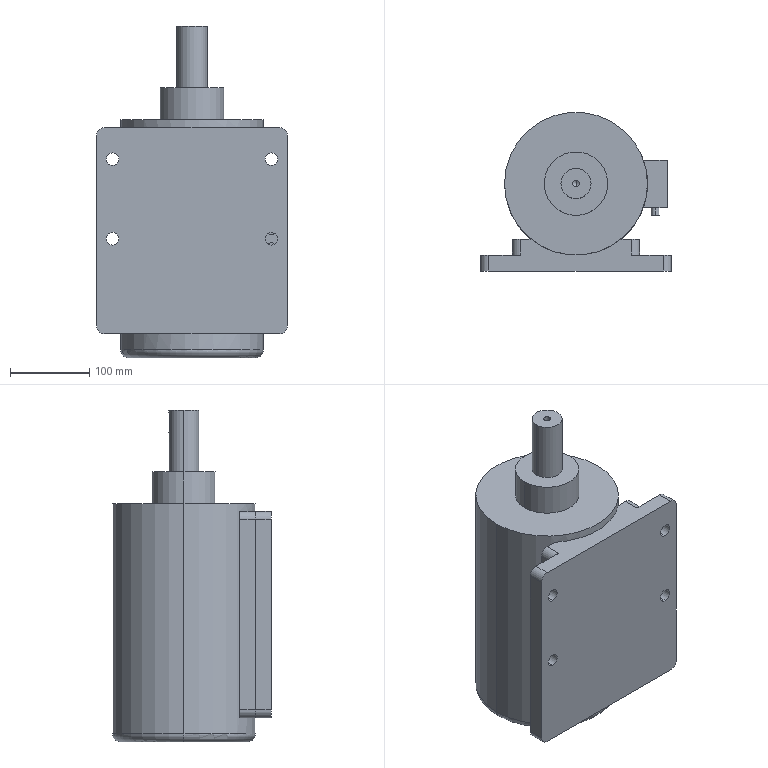Part | SolidWorks | 1 solid | 63 faces | box 240 x 200 x 417.5 mm | volume 9698693 mm3 | cylinder 33 | plane 26 | cone 2 | torus 2 | commonest cylinder face diameters 16 x8 20 x8 10 x6 12 x3 8.5 x2 38 x2